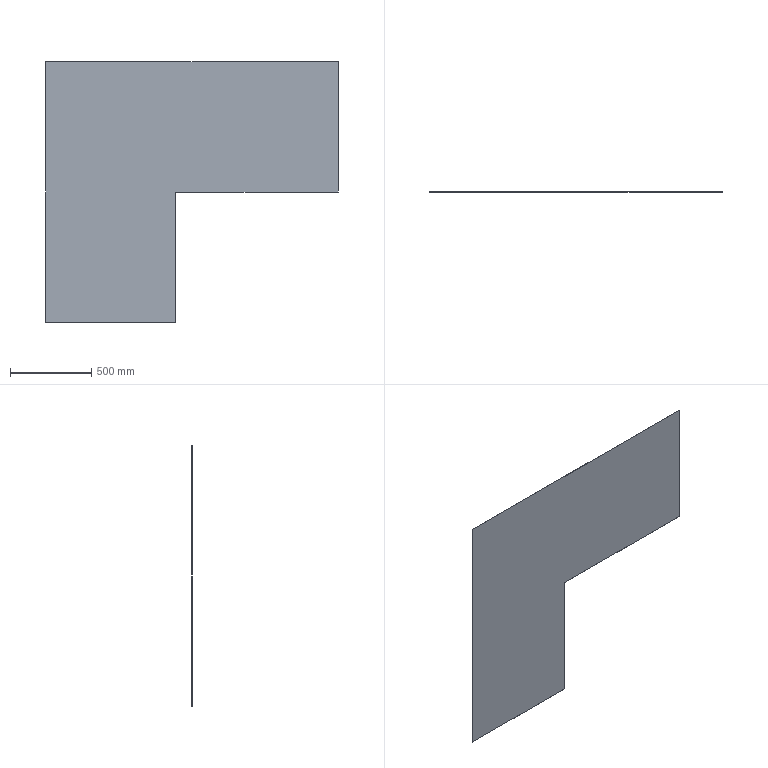Part | SolidWorks | features Extrusion 1 | 1 solid | 8 faces | box 1800 x 1 x 1600 mm | volume 2080000 mm3 | plane 8
STEP:
#1=CARTESIAN_POINT('',(-100.,0.,0.));
#2=VERTEX_POINT('',#1);
#3=CARTESIAN_POINT('',(-100.,0.,-800.));
#4=VERTEX_POINT('',#3);
#5=CARTESIAN_POINT('',(-100.,0.,-800.));
#6=DIRECTION('',(0.,0.,-1.));
#7=VECTOR('',#6,1000.);
#8=LINE('',#5,#7);
#9=EDGE_CURVE('',#2,#4,#8,.T.);
#10=ORIENTED_EDGE('',*,*,#9,.T.);
#11=CARTESIAN_POINT('',(-100.,1.,-800.));
#12=VERTEX_POINT('',#11);
#13=CARTESIAN_POINT('',(-100.,1.,-800.));
#14=DIRECTION('',(0.,-1.,0.));
#15=VECTOR('',#14,1000.);
#16=LINE('',#13,#15);
#17=EDGE_CURVE('',#12,#4,#16,.T.);
#18=ORIENTED_EDGE('',*,*,#17,.F.);
#19=CARTESIAN_POINT('',(-100.,1.,0.));
#20=VERTEX_POINT('',#19);
#21=CARTESIAN_POINT('',(-100.,1.,-800.));
#22=DIRECTION('',(0.,0.,-1.));
#23=VECTOR('',#22,1000.);
#24=LINE('',#21,#23);
#25=EDGE_CURVE('',#20,#12,#24,.T.);
#26=ORIENTED_EDGE('',*,*,#25,.F.);
#27=CARTESIAN_POINT('',(-100.,1.,0.));
#28=DIRECTION('',(0.,-1.,0.));
#29=VECTOR('',#28,1000.);
#30=LINE('',#27,#29);
#31=EDGE_CURVE('',#20,#2,#30,.T.);
#32=ORIENTED_EDGE('',*,*,#31,.T.);
#33=EDGE_LOOP('',(#10,#18,#26,#32));
#34=FACE_OUTER_BOUND('',#33,.T.);
#35=CARTESIAN_POINT('',(-100.,1.,-800.));
#36=DIRECTION('',(-1.,0.,0.));
#37=DIRECTION('',(0.,0.,1.));
#38=AXIS2_PLACEMENT_3D('',#35,#36,#37);
#39=PLANE('',#38);
#40=ADVANCED_FACE('',(#34),#39,.F.);
#41=CARTESIAN_POINT('',(-900.,0.,-800.));
#42=VERTEX_POINT('',#41);
#43=CARTESIAN_POINT('',(-900.,0.,-800.));
#44=DIRECTION('',(-1.,0.,0.));
#45=VECTOR('',#44,1000.);
#46=LINE('',#43,#45);
#47=EDGE_CURVE('',#4,#42,#46,.T.);
#48=ORIENTED_EDGE('',*,*,#47,.T.);
#49=CARTESIAN_POINT('',(-900.,1.,-800.));
#50=VERTEX_POINT('',#49);
#51=CARTESIAN_POINT('',(-900.,1.,-800.));
#52=DIRECTION('',(0.,-1.,0.));
#53=VECTOR('',#52,1000.);
#54=LINE('',#51,#53);
#55=EDGE_CURVE('',#50,#42,#54,.T.);
#56=ORIENTED_EDGE('',*,*,#55,.F.);
#57=CARTESIAN_POINT('',(-900.,1.,-800.));
#58=DIRECTION('',(-1.,0.,0.));
#59=VECTOR('',#58,1000.);
#60=LINE('',#57,#59);
#61=EDGE_CURVE('',#12,#50,#60,.T.);
#62=ORIENTED_EDGE('',*,*,#61,.F.);
#63=ORIENTED_EDGE('',*,*,#17,.T.);
#64=EDGE_LOOP('',(#48,#56,#62,#63));
#65=FACE_OUTER_BOUND('',#64,.T.);
#66=CARTESIAN_POINT('',(-900.,1.,-800.));
#67=DIRECTION('',(0.,0.,1.));
#68=DIRECTION('',(1.,0.,0.));
#69=AXIS2_PLACEMENT_3D('',#66,#67,#68);
#70=PLANE('',#69);
#71=ADVANCED_FACE('',(#65),#70,.F.);
#72=CARTESIAN_POINT('',(-900.,0.,800.));
#73=VERTEX_POINT('',#72);
#74=CARTESIAN_POINT('',(-900.,0.,800.));
#75=DIRECTION('',(0.,0.,1.));
#76=VECTOR('',#75,1000.);
#77=LINE('',#74,#76);
#78=EDGE_CURVE('',#42,#73,#77,.T.);
#79=ORIENTED_EDGE('',*,*,#78,.T.);
#80=CARTESIAN_POINT('',(-900.,1.,800.));
#81=VERTEX_POINT('',#80);
#82=CARTESIAN_POINT('',(-900.,1.,800.));
#83=DIRECTION('',(0.,-1.,0.));
#84=VECTOR('',#83,1000.);
#85=LINE('',#82,#84);
#86=EDGE_CURVE('',#81,#73,#85,.T.);
#87=ORIENTED_EDGE('',*,*,#86,.F.);
#88=CARTESIAN_POINT('',(-900.,1.,800.));
#89=DIRECTION('',(0.,0.,1.));
#90=VECTOR('',#89,1000.);
#91=LINE('',#88,#90);
#92=EDGE_CURVE('',#50,#81,#91,.T.);
#93=ORIENTED_EDGE('',*,*,#92,.F.);
#94=ORIENTED_EDGE('',*,*,#55,.T.);
#95=EDGE_LOOP('',(#79,#87,#93,#94));
#96=FACE_OUTER_BOUND('',#95,.T.);
#97=CARTESIAN_POINT('',(-900.,1.,800.));
#98=DIRECTION('',(1.,0.,0.));
#99=DIRECTION('',(0.,0.,-1.));
#100=AXIS2_PLACEMENT_3D('',#97,#98,#99);
#101=PLANE('',#100);
#102=ADVANCED_FACE('',(#96),#101,.F.);
#103=CARTESIAN_POINT('',(900.,0.,800.));
#104=VERTEX_POINT('',#103);
#105=CARTESIAN_POINT('',(-900.,0.,800.));
#106=DIRECTION('',(1.,0.,0.));
#107=VECTOR('',#106,1000.);
#108=LINE('',#105,#107);
#109=EDGE_CURVE('',#73,#104,#108,.T.);
#110=ORIENTED_EDGE('',*,*,#109,.T.);
#111=CARTESIAN_POINT('',(900.,1.,800.));
#112=VERTEX_POINT('',#111);
#113=CARTESIAN_POINT('',(900.,1.,800.));
#114=DIRECTION('',(0.,-1.,0.));
#115=VECTOR('',#114,1000.);
#116=LINE('',#113,#115);
#117=EDGE_CURVE('',#112,#104,#116,.T.);
#118=ORIENTED_EDGE('',*,*,#117,.F.);
#119=CARTESIAN_POINT('',(-900.,1.,800.));
#120=DIRECTION('',(1.,0.,0.));
#121=VECTOR('',#120,1000.);
#122=LINE('',#119,#121);
#123=EDGE_CURVE('',#81,#112,#122,.T.);
#124=ORIENTED_EDGE('',*,*,#123,.F.);
#125=ORIENTED_EDGE('',*,*,#86,.T.);
#126=EDGE_LOOP('',(#110,#118,#124,#125));
#127=FACE_OUTER_BOUND('',#126,.T.);
#128=CARTESIAN_POINT('',(-900.,1.,800.));
#129=DIRECTION('',(0.,0.,-1.));
#130=DIRECTION('',(-1.,0.,0.));
#131=AXIS2_PLACEMENT_3D('',#128,#129,#130);
#132=PLANE('',#131);
#133=ADVANCED_FACE('',(#127),#132,.F.);
#134=CARTESIAN_POINT('',(900.,0.,0.));
#135=VERTEX_POINT('',#134);
#136=CARTESIAN_POINT('',(900.,0.,800.));
#137=DIRECTION('',(0.,0.,-1.));
#138=VECTOR('',#137,1000.);
#139=LINE('',#136,#138);
#140=EDGE_CURVE('',#104,#135,#139,.T.);
#141=ORIENTED_EDGE('',*,*,#140,.T.);
#142=CARTESIAN_POINT('',(900.,1.,0.));
#143=VERTEX_POINT('',#142);
#144=CARTESIAN_POINT('',(900.,1.,0.));
#145=DIRECTION('',(0.,-1.,0.));
#146=VECTOR('',#145,1000.);
#147=LINE('',#144,#146);
#148=EDGE_CURVE('',#143,#135,#147,.T.);
#149=ORIENTED_EDGE('',*,*,#148,.F.);
#150=CARTESIAN_POINT('',(900.,1.,800.));
#151=DIRECTION('',(0.,0.,-1.));
#152=VECTOR('',#151,1000.);
#153=LINE('',#150,#152);
#154=EDGE_CURVE('',#112,#143,#153,.T.);
#155=ORIENTED_EDGE('',*,*,#154,.F.);
#156=ORIENTED_EDGE('',*,*,#117,.T.);
#157=EDGE_LOOP('',(#141,#149,#155,#156));
#158=FACE_OUTER_BOUND('',#157,.T.);
#159=CARTESIAN_POINT('',(900.,1.,800.));
#160=DIRECTION('',(-1.,0.,0.));
#161=DIRECTION('',(0.,0.,1.));
#162=AXIS2_PLACEMENT_3D('',#159,#160,#161);
#163=PLANE('',#162);
#164=ADVANCED_FACE('',(#158),#163,.F.);
#165=CARTESIAN_POINT('',(-100.,0.,0.));
#166=DIRECTION('',(-1.,0.,0.));
#167=VECTOR('',#166,1000.);
#168=LINE('',#165,#167);
#169=EDGE_CURVE('',#135,#2,#168,.T.);
#170=ORIENTED_EDGE('',*,*,#169,.T.);
#171=ORIENTED_EDGE('',*,*,#31,.F.);
#172=CARTESIAN_POINT('',(0.,1.,0.));
#173=DIRECTION('',(-1.,0.,0.));
#174=VECTOR('',#173,1000.);
#175=LINE('',#172,#174);
#176=EDGE_CURVE('',#143,#20,#175,.T.);
#177=ORIENTED_EDGE('',*,*,#176,.F.);
#178=ORIENTED_EDGE('',*,*,#148,.T.);
#179=EDGE_LOOP('',(#170,#171,#177,#178));
#180=FACE_OUTER_BOUND('',#179,.T.);
#181=CARTESIAN_POINT('',(-100.,1.,0.));
#182=DIRECTION('',(0.,0.,1.));
#183=DIRECTION('',(1.,0.,0.));
#184=AXIS2_PLACEMENT_3D('',#181,#182,#183);
#185=PLANE('',#184);
#186=ADVANCED_FACE('',(#180),#185,.F.);
#187=ORIENTED_EDGE('',*,*,#25,.T.);
#188=ORIENTED_EDGE('',*,*,#61,.T.);
#189=ORIENTED_EDGE('',*,*,#92,.T.);
#190=ORIENTED_EDGE('',*,*,#123,.T.);
#191=ORIENTED_EDGE('',*,*,#154,.T.);
#192=ORIENTED_EDGE('',*,*,#176,.T.);
#193=EDGE_LOOP('',(#187,#188,#189,#190,#191,#192));
#194=FACE_OUTER_BOUND('',#193,.T.);
#195=CARTESIAN_POINT('',(0.,1.,0.));
#196=DIRECTION('',(0.,1.,0.));
#197=DIRECTION('',(0.,0.,1.));
#198=AXIS2_PLACEMENT_3D('',#195,#196,#197);
#199=PLANE('',#198);
#200=ADVANCED_FACE('',(#194),#199,.T.);
#201=ORIENTED_EDGE('',*,*,#9,.F.);
#202=ORIENTED_EDGE('',*,*,#169,.F.);
#203=ORIENTED_EDGE('',*,*,#140,.F.);
#204=ORIENTED_EDGE('',*,*,#109,.F.);
#205=ORIENTED_EDGE('',*,*,#78,.F.);
#206=ORIENTED_EDGE('',*,*,#47,.F.);
#207=EDGE_LOOP('',(#201,#202,#203,#204,#205,#206));
#208=FACE_OUTER_BOUND('',#207,.T.);
#209=CARTESIAN_POINT('',(0.,0.,0.));
#210=DIRECTION('',(0.,1.,0.));
#211=DIRECTION('',(0.,0.,1.));
#212=AXIS2_PLACEMENT_3D('',#209,#210,#211);
#213=PLANE('',#212);
#214=ADVANCED_FACE('',(#208),#213,.F.);
#215=CLOSED_SHELL('',(#40,#71,#102,#133,#164,#186,#200,#214));
#216=MANIFOLD_SOLID_BREP('',#215);
#217=CARTESIAN_POINT('',(0.,0.,0.));
#218=DIRECTION('',(0.,0.,1.));
#219=DIRECTION('',(1.,0.,0.));
#220=AXIS2_PLACEMENT_3D('',#217,#218,#219);
#221=(LENGTH_UNIT()NAMED_UNIT(*)SI_UNIT(.MILLI.,.METRE.));
#222=UNCERTAINTY_MEASURE_WITH_UNIT(LENGTH_MEASURE(0.00001),#221,'','');
#223=(NAMED_UNIT(*)PLANE_ANGLE_UNIT()SI_UNIT($,.RADIAN.));
#224=(NAMED_UNIT(*)SI_UNIT($,.STERADIAN.)SOLID_ANGLE_UNIT());
#225=(GEOMETRIC_REPRESENTATION_CONTEXT(3)GLOBAL_UNCERTAINTY_ASSIGNED_CONTEXT((#222))GLOBAL_UNIT_ASSIGNED_CONTEXT((#221,#223,#224))REPRESENTATION_CONTEXT('',''));
#226=ADVANCED_BREP_SHAPE_REPRESENTATION('',(#216,#220),#225);